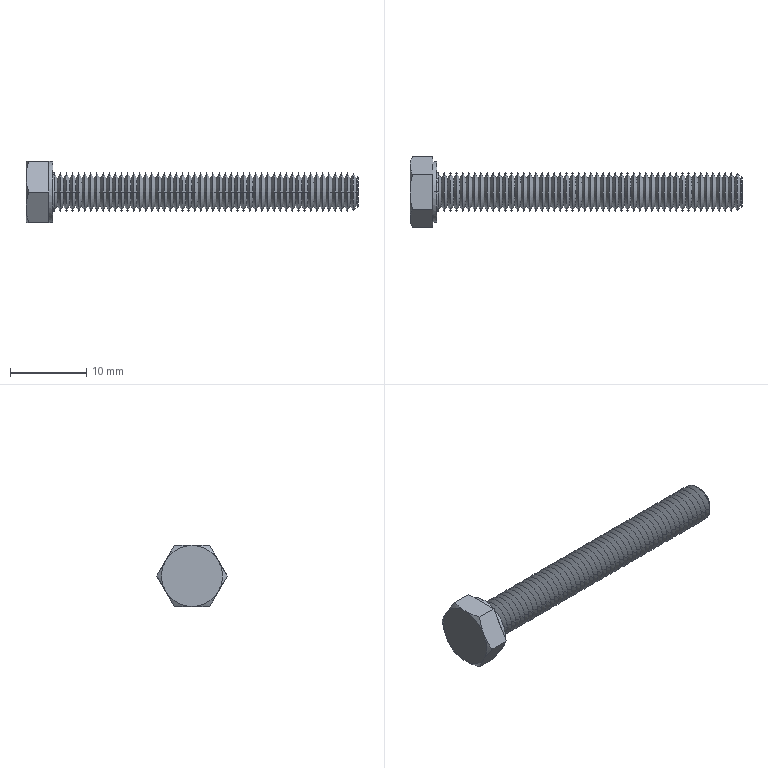Part | SolidWorks | features RevCut 4, Chamfer 1, Extrusion 1, Fillet 1, LPattern 1, Revolution 1 | 1 solid | 325 faces | box 43.5 x 9.238 x 8 mm | volume 779.159 mm3 | cone 210 | cylinder 98 | plane 15 | torus 2 | commonest cylinder face diameters 5 x96 8 x2